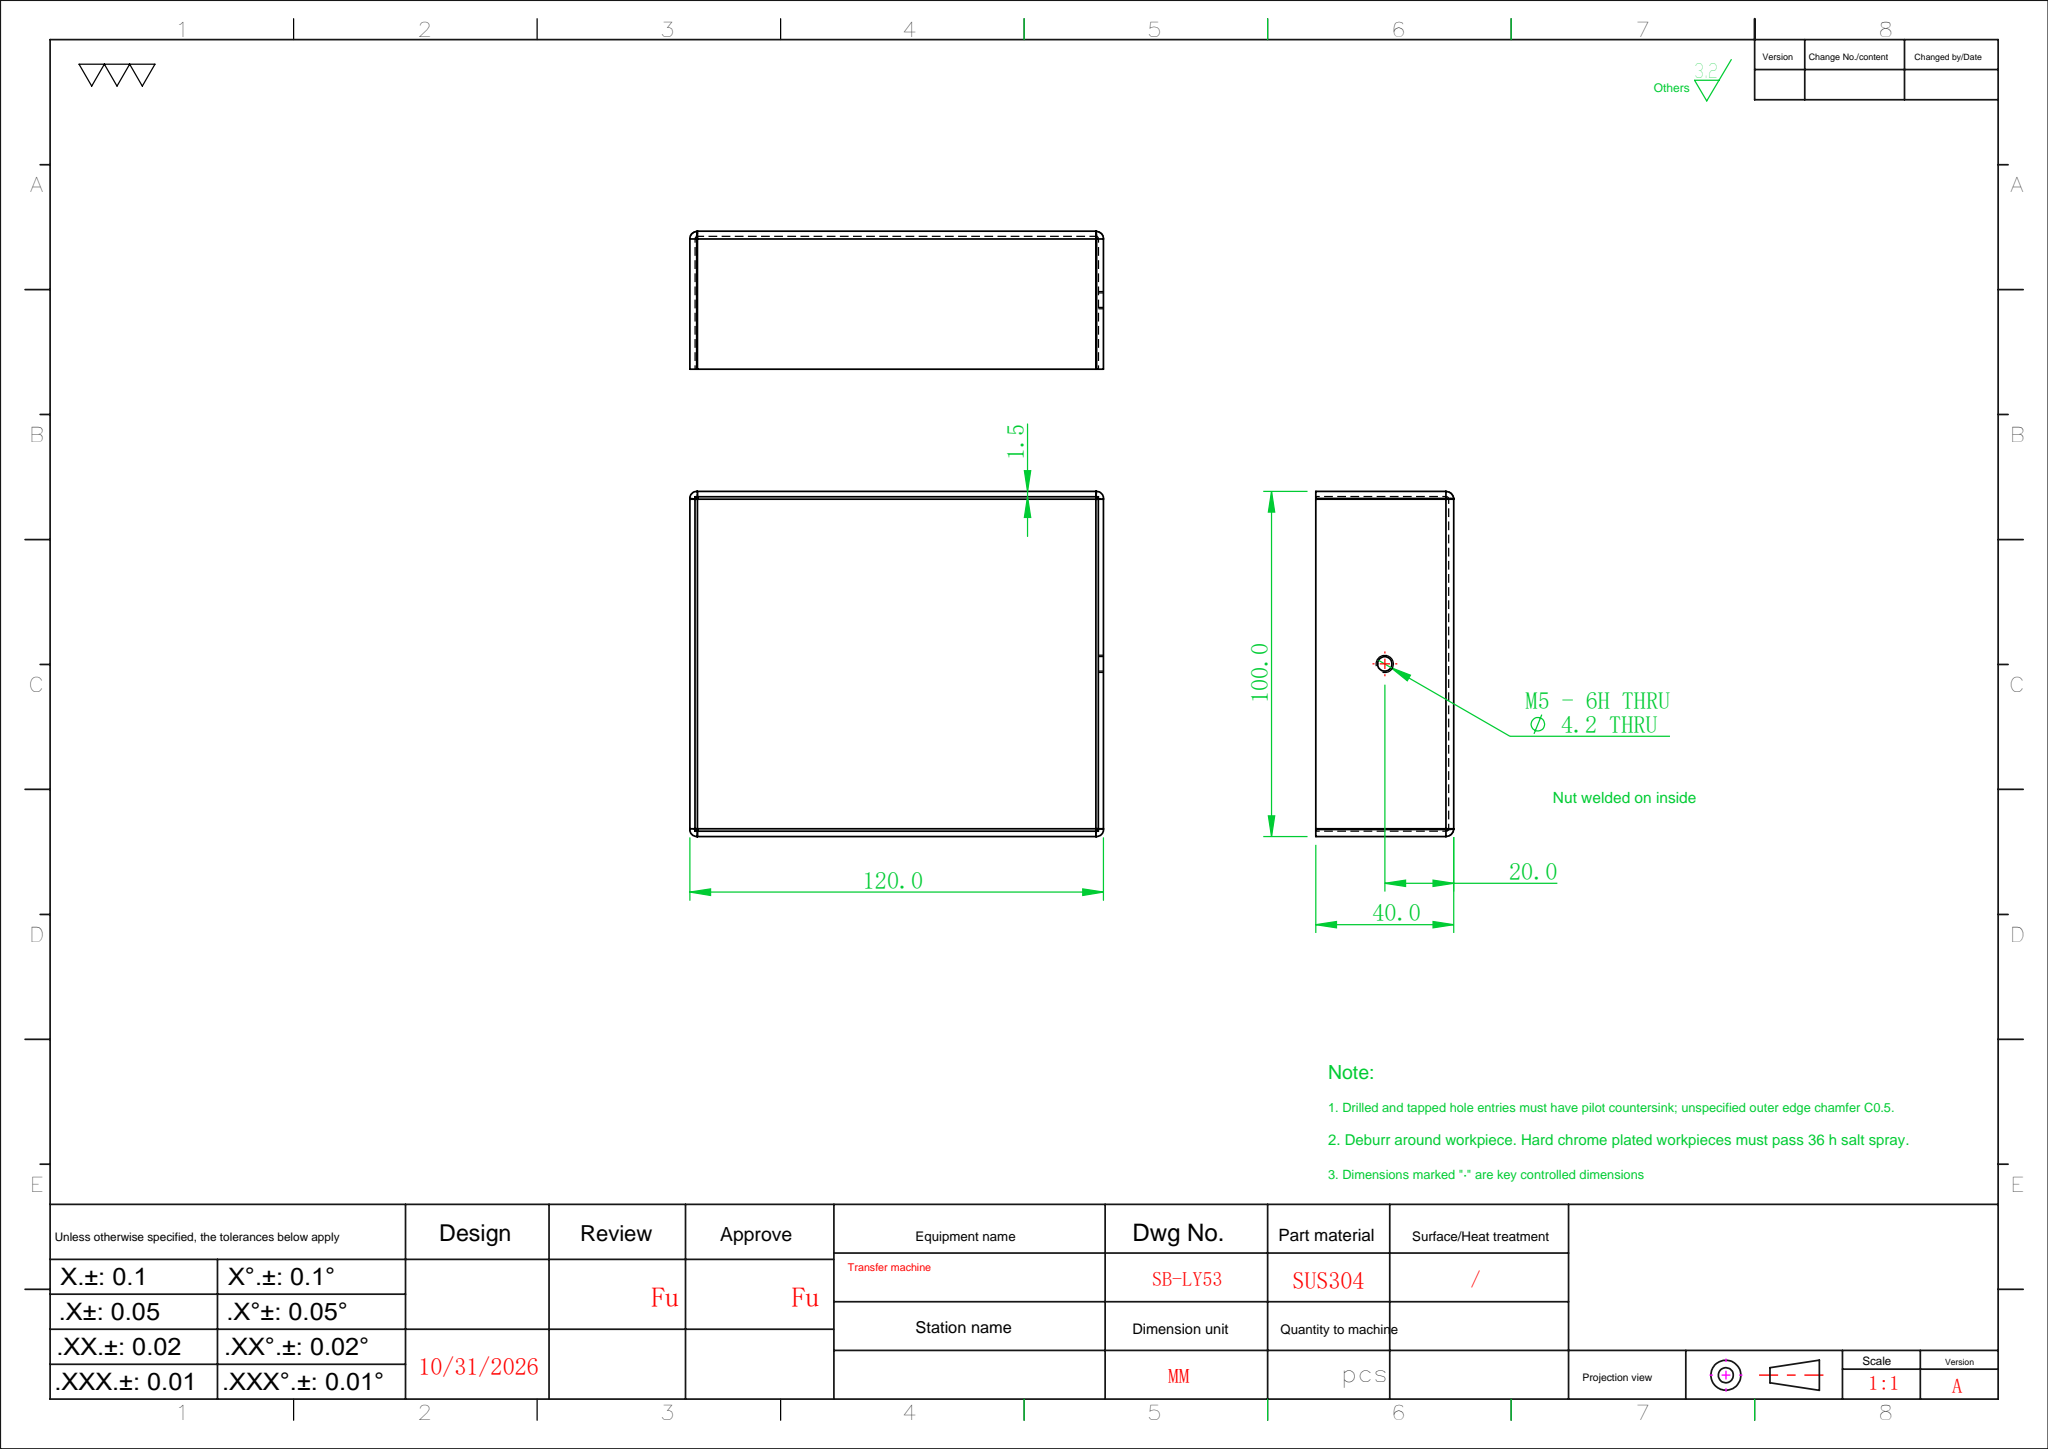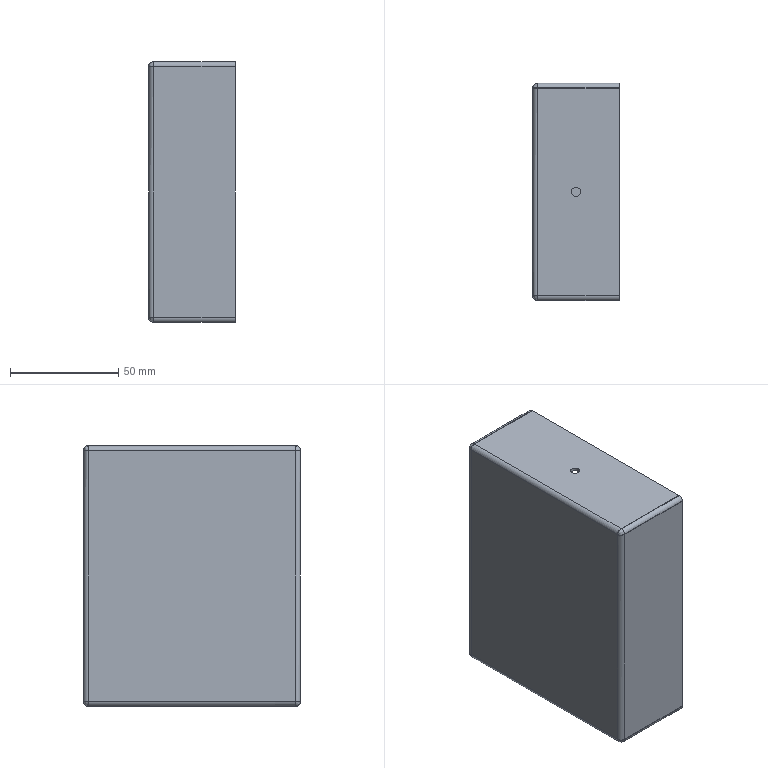Part | SolidWorks | features SMWeldBead 4, EdgeFlange 1, FlatPattern 1, HoleWzd 1, SMBaseFlange 1, SheetMetal 1 | 1 solid | 68 faces | box 40 x 100 x 120 mm | volume 42493 mm3 | plane 34 | spline 20 | cylinder 14 | commonest cylinder face diameters 1.473 x4 4 x4 4.473 x4 4.2 x2